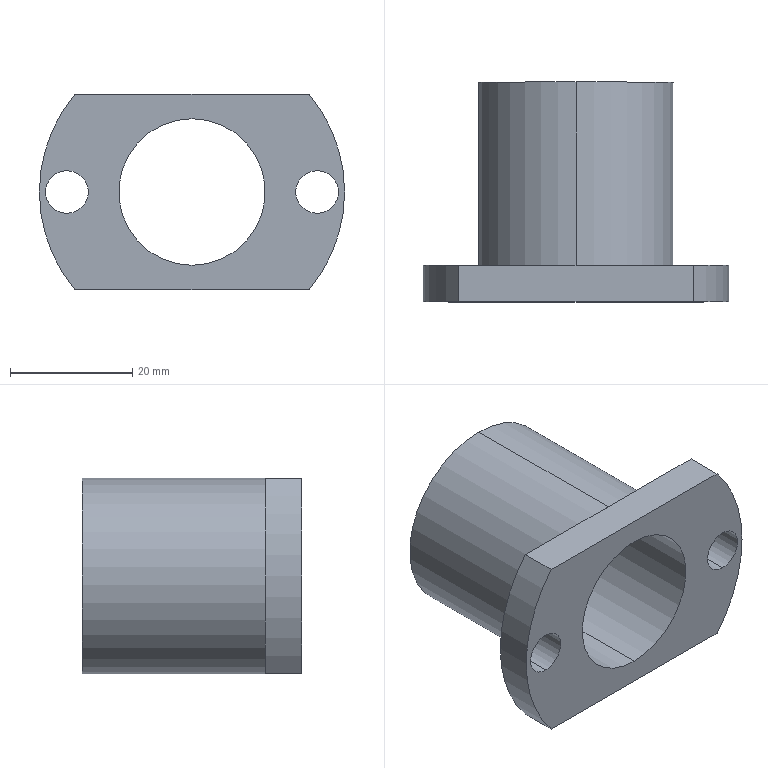Part | SolidWorks | features ICE 2, Revolution 1 | 1 solid | 16 faces | box 50 x 36 x 32 mm | volume 16277 mm3 | cylinder 10 | plane 6 | commonest cylinder face diameters 7 x4 24 x2 32 x2 50 x2
STEP:
#1=CARTESIAN_POINT('',(20.5,0.,-3.5));
#2=VERTEX_POINT('',#1);
#3=CARTESIAN_POINT('',(20.5,0.,3.5));
#4=VERTEX_POINT('',#3);
#5=CARTESIAN_POINT('',(20.5,0.,0.));
#6=DIRECTION('',(0.,1.,0.));
#7=DIRECTION('',(0.,0.,1.));
#8=AXIS2_PLACEMENT_3D('',#5,#6,#7);
#9=CIRCLE('',#8,3.5);
#10=EDGE_CURVE('',#2,#4,#9,.T.);
#11=ORIENTED_EDGE('',*,*,#10,.F.);
#12=CARTESIAN_POINT('',(20.5,6.,-3.5));
#13=VERTEX_POINT('',#12);
#14=CARTESIAN_POINT('',(20.5,0.,-3.5));
#15=DIRECTION('',(0.,1.,0.));
#16=VECTOR('',#15,1000.);
#17=LINE('',#14,#16);
#18=EDGE_CURVE('',#2,#13,#17,.T.);
#19=ORIENTED_EDGE('',*,*,#18,.T.);
#20=CARTESIAN_POINT('',(20.5,6.,3.5));
#21=VERTEX_POINT('',#20);
#22=CARTESIAN_POINT('',(20.5,6.,0.));
#23=DIRECTION('',(0.,1.,0.));
#24=DIRECTION('',(0.,0.,1.));
#25=AXIS2_PLACEMENT_3D('',#22,#23,#24);
#26=CIRCLE('',#25,3.5);
#27=EDGE_CURVE('',#13,#21,#26,.T.);
#28=ORIENTED_EDGE('',*,*,#27,.T.);
#29=CARTESIAN_POINT('',(20.5,0.,3.5));
#30=DIRECTION('',(0.,1.,0.));
#31=VECTOR('',#30,1000.);
#32=LINE('',#29,#31);
#33=EDGE_CURVE('',#4,#21,#32,.T.);
#34=ORIENTED_EDGE('',*,*,#33,.F.);
#35=EDGE_LOOP('',(#11,#19,#28,#34));
#36=FACE_OUTER_BOUND('',#35,.T.);
#37=CARTESIAN_POINT('',(20.5,0.,0.));
#38=DIRECTION('',(0.,1.,0.));
#39=DIRECTION('',(0.,0.,1.));
#40=AXIS2_PLACEMENT_3D('',#37,#38,#39);
#41=CYLINDRICAL_SURFACE('',#40,3.5);
#42=ADVANCED_FACE('',(#36),#41,.F.);
#43=CARTESIAN_POINT('',(-20.5,0.,-3.5));
#44=VERTEX_POINT('',#43);
#45=CARTESIAN_POINT('',(-20.5,0.,3.5));
#46=VERTEX_POINT('',#45);
#47=CARTESIAN_POINT('',(-20.5,0.,0.));
#48=DIRECTION('',(0.,1.,0.));
#49=DIRECTION('',(0.,0.,1.));
#50=AXIS2_PLACEMENT_3D('',#47,#48,#49);
#51=CIRCLE('',#50,3.5);
#52=EDGE_CURVE('',#44,#46,#51,.T.);
#53=ORIENTED_EDGE('',*,*,#52,.F.);
#54=CARTESIAN_POINT('',(-20.5,6.,-3.5));
#55=VERTEX_POINT('',#54);
#56=CARTESIAN_POINT('',(-20.5,0.,-3.5));
#57=DIRECTION('',(0.,1.,0.));
#58=VECTOR('',#57,1000.);
#59=LINE('',#56,#58);
#60=EDGE_CURVE('',#44,#55,#59,.T.);
#61=ORIENTED_EDGE('',*,*,#60,.T.);
#62=CARTESIAN_POINT('',(-20.5,6.,3.5));
#63=VERTEX_POINT('',#62);
#64=CARTESIAN_POINT('',(-20.5,6.,0.));
#65=DIRECTION('',(0.,1.,0.));
#66=DIRECTION('',(0.,0.,1.));
#67=AXIS2_PLACEMENT_3D('',#64,#65,#66);
#68=CIRCLE('',#67,3.5);
#69=EDGE_CURVE('',#55,#63,#68,.T.);
#70=ORIENTED_EDGE('',*,*,#69,.T.);
#71=CARTESIAN_POINT('',(-20.5,0.,3.5));
#72=DIRECTION('',(0.,1.,0.));
#73=VECTOR('',#72,1000.);
#74=LINE('',#71,#73);
#75=EDGE_CURVE('',#46,#63,#74,.T.);
#76=ORIENTED_EDGE('',*,*,#75,.F.);
#77=EDGE_LOOP('',(#53,#61,#70,#76));
#78=FACE_OUTER_BOUND('',#77,.T.);
#79=CARTESIAN_POINT('',(-20.5,0.,0.));
#80=DIRECTION('',(0.,1.,0.));
#81=DIRECTION('',(0.,0.,1.));
#82=AXIS2_PLACEMENT_3D('',#79,#80,#81);
#83=CYLINDRICAL_SURFACE('',#82,3.5);
#84=ADVANCED_FACE('',(#78),#83,.F.);
#85=CARTESIAN_POINT('',(0.,36.,-16.));
#86=VERTEX_POINT('',#85);
#87=CARTESIAN_POINT('',(0.,36.,16.));
#88=VERTEX_POINT('',#87);
#89=CARTESIAN_POINT('',(0.,36.,0.));
#90=DIRECTION('',(0.,-1.,0.));
#91=DIRECTION('',(0.,0.,-1.));
#92=AXIS2_PLACEMENT_3D('',#89,#90,#91);
#93=CIRCLE('',#92,16.);
#94=EDGE_CURVE('',#86,#88,#93,.T.);
#95=ORIENTED_EDGE('',*,*,#94,.T.);
#96=CARTESIAN_POINT('',(0.,6.,16.));
#97=VERTEX_POINT('',#96);
#98=CARTESIAN_POINT('',(0.,0.,16.));
#99=DIRECTION('',(0.,-1.,0.));
#100=VECTOR('',#99,1000.);
#101=LINE('',#98,#100);
#102=EDGE_CURVE('',#88,#97,#101,.T.);
#103=ORIENTED_EDGE('',*,*,#102,.T.);
#104=CARTESIAN_POINT('',(0.,6.,-16.));
#105=VERTEX_POINT('',#104);
#106=CARTESIAN_POINT('',(0.,6.,0.));
#107=DIRECTION('',(0.,-1.,0.));
#108=DIRECTION('',(0.,0.,-1.));
#109=AXIS2_PLACEMENT_3D('',#106,#107,#108);
#110=CIRCLE('',#109,16.);
#111=EDGE_CURVE('',#105,#97,#110,.T.);
#112=ORIENTED_EDGE('',*,*,#111,.F.);
#113=CARTESIAN_POINT('',(0.,0.,-16.));
#114=DIRECTION('',(0.,-1.,0.));
#115=VECTOR('',#114,1000.);
#116=LINE('',#113,#115);
#117=EDGE_CURVE('',#86,#105,#116,.T.);
#118=ORIENTED_EDGE('',*,*,#117,.F.);
#119=EDGE_LOOP('',(#95,#103,#112,#118));
#120=FACE_OUTER_BOUND('',#119,.T.);
#121=CARTESIAN_POINT('',(0.,0.,0.));
#122=DIRECTION('',(0.,-1.,0.));
#123=DIRECTION('',(0.,0.,-1.));
#124=AXIS2_PLACEMENT_3D('',#121,#122,#123);
#125=CYLINDRICAL_SURFACE('',#124,16.);
#126=ADVANCED_FACE('',(#120),#125,.T.);
#127=CARTESIAN_POINT('',(0.,36.,12.));
#128=VERTEX_POINT('',#127);
#129=CARTESIAN_POINT('',(0.,36.,-12.));
#130=VERTEX_POINT('',#129);
#131=CARTESIAN_POINT('',(0.,36.,0.));
#132=DIRECTION('',(0.,-1.,0.));
#133=DIRECTION('',(0.,0.,-1.));
#134=AXIS2_PLACEMENT_3D('',#131,#132,#133);
#135=CIRCLE('',#134,12.);
#136=EDGE_CURVE('',#128,#130,#135,.T.);
#137=ORIENTED_EDGE('',*,*,#136,.F.);
#138=CARTESIAN_POINT('',(0.,0.,12.));
#139=VERTEX_POINT('',#138);
#140=CARTESIAN_POINT('',(0.,0.,12.));
#141=DIRECTION('',(0.,-1.,0.));
#142=VECTOR('',#141,1000.);
#143=LINE('',#140,#142);
#144=EDGE_CURVE('',#128,#139,#143,.T.);
#145=ORIENTED_EDGE('',*,*,#144,.T.);
#146=CARTESIAN_POINT('',(0.,0.,-12.));
#147=VERTEX_POINT('',#146);
#148=CARTESIAN_POINT('',(0.,0.,0.));
#149=DIRECTION('',(0.,-1.,0.));
#150=DIRECTION('',(0.,0.,-1.));
#151=AXIS2_PLACEMENT_3D('',#148,#149,#150);
#152=CIRCLE('',#151,12.);
#153=EDGE_CURVE('',#139,#147,#152,.T.);
#154=ORIENTED_EDGE('',*,*,#153,.T.);
#155=CARTESIAN_POINT('',(0.,0.,-12.));
#156=DIRECTION('',(0.,-1.,0.));
#157=VECTOR('',#156,1000.);
#158=LINE('',#155,#157);
#159=EDGE_CURVE('',#130,#147,#158,.T.);
#160=ORIENTED_EDGE('',*,*,#159,.F.);
#161=EDGE_LOOP('',(#137,#145,#154,#160));
#162=FACE_OUTER_BOUND('',#161,.T.);
#163=CARTESIAN_POINT('',(0.,0.,0.));
#164=DIRECTION('',(0.,-1.,0.));
#165=DIRECTION('',(0.,0.,-1.));
#166=AXIS2_PLACEMENT_3D('',#163,#164,#165);
#167=CYLINDRICAL_SURFACE('',#166,12.);
#168=ADVANCED_FACE('',(#162),#167,.F.);
#169=CARTESIAN_POINT('',(19.209,0.,16.));
#170=VERTEX_POINT('',#169);
#171=CARTESIAN_POINT('',(19.209,6.,16.));
#172=VERTEX_POINT('',#171);
#173=CARTESIAN_POINT('',(19.209,0.,16.));
#174=DIRECTION('',(0.,1.,0.));
#175=VECTOR('',#174,1000.);
#176=LINE('',#173,#175);
#177=EDGE_CURVE('',#170,#172,#176,.T.);
#178=ORIENTED_EDGE('',*,*,#177,.F.);
#179=CARTESIAN_POINT('',(19.209,0.,-16.));
#180=VERTEX_POINT('',#179);
#181=CARTESIAN_POINT('',(0.,0.,0.));
#182=DIRECTION('',(0.,-1.,0.));
#183=DIRECTION('',(0.,0.,-1.));
#184=AXIS2_PLACEMENT_3D('',#181,#182,#183);
#185=CIRCLE('',#184,25.);
#186=EDGE_CURVE('',#180,#170,#185,.T.);
#187=ORIENTED_EDGE('',*,*,#186,.F.);
#188=CARTESIAN_POINT('',(19.209,6.,-16.));
#189=VERTEX_POINT('',#188);
#190=CARTESIAN_POINT('',(19.209,0.,-16.));
#191=DIRECTION('',(0.,1.,0.));
#192=VECTOR('',#191,1000.);
#193=LINE('',#190,#192);
#194=EDGE_CURVE('',#180,#189,#193,.T.);
#195=ORIENTED_EDGE('',*,*,#194,.T.);
#196=CARTESIAN_POINT('',(0.,6.,0.));
#197=DIRECTION('',(0.,-1.,0.));
#198=DIRECTION('',(0.,0.,-1.));
#199=AXIS2_PLACEMENT_3D('',#196,#197,#198);
#200=CIRCLE('',#199,25.);
#201=EDGE_CURVE('',#189,#172,#200,.T.);
#202=ORIENTED_EDGE('',*,*,#201,.T.);
#203=EDGE_LOOP('',(#178,#187,#195,#202));
#204=FACE_OUTER_BOUND('',#203,.T.);
#205=CARTESIAN_POINT('',(0.,0.,0.));
#206=DIRECTION('',(0.,-1.,0.));
#207=DIRECTION('',(0.,0.,-1.));
#208=AXIS2_PLACEMENT_3D('',#205,#206,#207);
#209=CYLINDRICAL_SURFACE('',#208,25.);
#210=ADVANCED_FACE('',(#204),#209,.T.);
#211=CARTESIAN_POINT('',(-19.209,6.,16.));
#212=DIRECTION('',(-1.,0.,0.));
#213=VECTOR('',#212,1000.);
#214=LINE('',#211,#213);
#215=EDGE_CURVE('',#172,#97,#214,.T.);
#216=ORIENTED_EDGE('',*,*,#215,.F.);
#217=ORIENTED_EDGE('',*,*,#201,.F.);
#218=CARTESIAN_POINT('',(-19.209,6.,-16.));
#219=DIRECTION('',(1.,0.,0.));
#220=VECTOR('',#219,1000.);
#221=LINE('',#218,#220);
#222=EDGE_CURVE('',#105,#189,#221,.T.);
#223=ORIENTED_EDGE('',*,*,#222,.F.);
#224=ORIENTED_EDGE('',*,*,#111,.T.);
#225=EDGE_LOOP('',(#216,#217,#223,#224));
#226=FACE_OUTER_BOUND('',#225,.T.);
#227=CARTESIAN_POINT('',(20.5,6.,0.));
#228=DIRECTION('',(0.,1.,0.));
#229=DIRECTION('',(0.,0.,1.));
#230=AXIS2_PLACEMENT_3D('',#227,#228,#229);
#231=CIRCLE('',#230,3.5);
#232=EDGE_CURVE('',#21,#13,#231,.T.);
#233=ORIENTED_EDGE('',*,*,#232,.F.);
#234=ORIENTED_EDGE('',*,*,#27,.F.);
#235=EDGE_LOOP('',(#233,#234));
#236=FACE_BOUND('',#235,.T.);
#237=CARTESIAN_POINT('',(25.,6.,0.));
#238=DIRECTION('',(0.,1.,0.));
#239=DIRECTION('',(0.,0.,1.));
#240=AXIS2_PLACEMENT_3D('',#237,#238,#239);
#241=PLANE('',#240);
#242=ADVANCED_FACE('',(#226,#236),#241,.T.);
#243=CARTESIAN_POINT('',(0.,36.,0.));
#244=DIRECTION('',(0.,-1.,0.));
#245=DIRECTION('',(0.,0.,-1.));
#246=AXIS2_PLACEMENT_3D('',#243,#244,#245);
#247=CIRCLE('',#246,12.);
#248=EDGE_CURVE('',#130,#128,#247,.T.);
#249=ORIENTED_EDGE('',*,*,#248,.T.);
#250=ORIENTED_EDGE('',*,*,#136,.T.);
#251=EDGE_LOOP('',(#249,#250));
#252=FACE_BOUND('',#251,.T.);
#253=ORIENTED_EDGE('',*,*,#94,.F.);
#254=CARTESIAN_POINT('',(0.,36.,0.));
#255=DIRECTION('',(0.,-1.,0.));
#256=DIRECTION('',(0.,0.,-1.));
#257=AXIS2_PLACEMENT_3D('',#254,#255,#256);
#258=CIRCLE('',#257,16.);
#259=EDGE_CURVE('',#88,#86,#258,.T.);
#260=ORIENTED_EDGE('',*,*,#259,.F.);
#261=EDGE_LOOP('',(#253,#260));
#262=FACE_OUTER_BOUND('',#261,.T.);
#263=CARTESIAN_POINT('',(16.,36.,0.));
#264=DIRECTION('',(0.,1.,0.));
#265=DIRECTION('',(0.,0.,1.));
#266=AXIS2_PLACEMENT_3D('',#263,#264,#265);
#267=PLANE('',#266);
#268=ADVANCED_FACE('',(#252,#262),#267,.T.);
#269=ORIENTED_EDGE('',*,*,#144,.F.);
#270=ORIENTED_EDGE('',*,*,#248,.F.);
#271=ORIENTED_EDGE('',*,*,#159,.T.);
#272=CARTESIAN_POINT('',(0.,0.,0.));
#273=DIRECTION('',(0.,-1.,0.));
#274=DIRECTION('',(0.,0.,-1.));
#275=AXIS2_PLACEMENT_3D('',#272,#273,#274);
#276=CIRCLE('',#275,12.);
#277=EDGE_CURVE('',#147,#139,#276,.T.);
#278=ORIENTED_EDGE('',*,*,#277,.T.);
#279=EDGE_LOOP('',(#269,#270,#271,#278));
#280=FACE_OUTER_BOUND('',#279,.T.);
#281=CARTESIAN_POINT('',(0.,0.,0.));
#282=DIRECTION('',(0.,-1.,0.));
#283=DIRECTION('',(0.,0.,-1.));
#284=AXIS2_PLACEMENT_3D('',#281,#282,#283);
#285=CYLINDRICAL_SURFACE('',#284,12.);
#286=ADVANCED_FACE('',(#280),#285,.F.);
#287=CARTESIAN_POINT('',(-19.209,0.,16.));
#288=VERTEX_POINT('',#287);
#289=CARTESIAN_POINT('',(-19.209,0.,16.));
#290=DIRECTION('',(-1.,0.,0.));
#291=VECTOR('',#290,1000.);
#292=LINE('',#289,#291);
#293=EDGE_CURVE('',#170,#288,#292,.T.);
#294=ORIENTED_EDGE('',*,*,#293,.T.);
#295=CARTESIAN_POINT('',(-19.209,0.,-16.));
#296=VERTEX_POINT('',#295);
#297=CARTESIAN_POINT('',(0.,0.,0.));
#298=DIRECTION('',(0.,-1.,0.));
#299=DIRECTION('',(0.,0.,-1.));
#300=AXIS2_PLACEMENT_3D('',#297,#298,#299);
#301=CIRCLE('',#300,25.);
#302=EDGE_CURVE('',#288,#296,#301,.T.);
#303=ORIENTED_EDGE('',*,*,#302,.T.);
#304=CARTESIAN_POINT('',(-19.209,0.,-16.));
#305=DIRECTION('',(1.,0.,0.));
#306=VECTOR('',#305,1000.);
#307=LINE('',#304,#306);
#308=EDGE_CURVE('',#296,#180,#307,.T.);
#309=ORIENTED_EDGE('',*,*,#308,.T.);
#310=ORIENTED_EDGE('',*,*,#186,.T.);
#311=EDGE_LOOP('',(#294,#303,#309,#310));
#312=FACE_OUTER_BOUND('',#311,.T.);
#313=CARTESIAN_POINT('',(20.5,0.,0.));
#314=DIRECTION('',(0.,1.,0.));
#315=DIRECTION('',(0.,0.,1.));
#316=AXIS2_PLACEMENT_3D('',#313,#314,#315);
#317=CIRCLE('',#316,3.5);
#318=EDGE_CURVE('',#4,#2,#317,.T.);
#319=ORIENTED_EDGE('',*,*,#318,.T.);
#320=ORIENTED_EDGE('',*,*,#10,.T.);
#321=EDGE_LOOP('',(#319,#320));
#322=FACE_BOUND('',#321,.T.);
#323=CARTESIAN_POINT('',(-20.5,0.,0.));
#324=DIRECTION('',(0.,1.,0.));
#325=DIRECTION('',(0.,0.,1.));
#326=AXIS2_PLACEMENT_3D('',#323,#324,#325);
#327=CIRCLE('',#326,3.5);
#328=EDGE_CURVE('',#46,#44,#327,.T.);
#329=ORIENTED_EDGE('',*,*,#328,.T.);
#330=ORIENTED_EDGE('',*,*,#52,.T.);
#331=EDGE_LOOP('',(#329,#330));
#332=FACE_BOUND('',#331,.T.);
#333=ORIENTED_EDGE('',*,*,#277,.F.);
#334=ORIENTED_EDGE('',*,*,#153,.F.);
#335=EDGE_LOOP('',(#333,#334));
#336=FACE_BOUND('',#335,.T.);
#337=CARTESIAN_POINT('',(12.,0.,0.));
#338=DIRECTION('',(0.,-1.,0.));
#339=DIRECTION('',(0.,0.,-1.));
#340=AXIS2_PLACEMENT_3D('',#337,#338,#339);
#341=PLANE('',#340);
#342=ADVANCED_FACE('',(#312,#322,#332,#336),#341,.T.);
#343=CARTESIAN_POINT('',(-19.209,6.,16.));
#344=VERTEX_POINT('',#343);
#345=CARTESIAN_POINT('',(-19.209,0.,16.));
#346=DIRECTION('',(0.,1.,0.));
#347=VECTOR('',#346,1000.);
#348=LINE('',#345,#347);
#349=EDGE_CURVE('',#288,#344,#348,.T.);
#350=ORIENTED_EDGE('',*,*,#349,.T.);
#351=CARTESIAN_POINT('',(-19.209,6.,-16.));
#352=VERTEX_POINT('',#351);
#353=CARTESIAN_POINT('',(0.,6.,0.));
#354=DIRECTION('',(0.,-1.,0.));
#355=DIRECTION('',(0.,0.,-1.));
#356=AXIS2_PLACEMENT_3D('',#353,#354,#355);
#357=CIRCLE('',#356,25.);
#358=EDGE_CURVE('',#344,#352,#357,.T.);
#359=ORIENTED_EDGE('',*,*,#358,.T.);
#360=CARTESIAN_POINT('',(-19.209,0.,-16.));
#361=DIRECTION('',(0.,1.,0.));
#362=VECTOR('',#361,1000.);
#363=LINE('',#360,#362);
#364=EDGE_CURVE('',#296,#352,#363,.T.);
#365=ORIENTED_EDGE('',*,*,#364,.F.);
#366=ORIENTED_EDGE('',*,*,#302,.F.);
#367=EDGE_LOOP('',(#350,#359,#365,#366));
#368=FACE_OUTER_BOUND('',#367,.T.);
#369=CARTESIAN_POINT('',(0.,0.,0.));
#370=DIRECTION('',(0.,-1.,0.));
#371=DIRECTION('',(0.,0.,-1.));
#372=AXIS2_PLACEMENT_3D('',#369,#370,#371);
#373=CYLINDRICAL_SURFACE('',#372,25.);
#374=ADVANCED_FACE('',(#368),#373,.T.);
#375=CARTESIAN_POINT('',(-19.209,6.,16.));
#376=DIRECTION('',(-1.,0.,0.));
#377=VECTOR('',#376,1000.);
#378=LINE('',#375,#377);
#379=EDGE_CURVE('',#97,#344,#378,.T.);
#380=ORIENTED_EDGE('',*,*,#379,.F.);
#381=CARTESIAN_POINT('',(0.,6.,0.));
#382=DIRECTION('',(0.,-1.,0.));
#383=DIRECTION('',(0.,0.,-1.));
#384=AXIS2_PLACEMENT_3D('',#381,#382,#383);
#385=CIRCLE('',#384,16.);
#386=EDGE_CURVE('',#97,#105,#385,.T.);
#387=ORIENTED_EDGE('',*,*,#386,.T.);
#388=CARTESIAN_POINT('',(-19.209,6.,-16.));
#389=DIRECTION('',(1.,0.,0.));
#390=VECTOR('',#389,1000.);
#391=LINE('',#388,#390);
#392=EDGE_CURVE('',#352,#105,#391,.T.);
#393=ORIENTED_EDGE('',*,*,#392,.F.);
#394=ORIENTED_EDGE('',*,*,#358,.F.);
#395=EDGE_LOOP('',(#380,#387,#393,#394));
#396=FACE_OUTER_BOUND('',#395,.T.);
#397=CARTESIAN_POINT('',(-20.5,6.,0.));
#398=DIRECTION('',(0.,1.,0.));
#399=DIRECTION('',(0.,0.,1.));
#400=AXIS2_PLACEMENT_3D('',#397,#398,#399);
#401=CIRCLE('',#400,3.5);
#402=EDGE_CURVE('',#63,#55,#401,.T.);
#403=ORIENTED_EDGE('',*,*,#402,.F.);
#404=ORIENTED_EDGE('',*,*,#69,.F.);
#405=EDGE_LOOP('',(#403,#404));
#406=FACE_BOUND('',#405,.T.);
#407=CARTESIAN_POINT('',(25.,6.,0.));
#408=DIRECTION('',(0.,1.,0.));
#409=DIRECTION('',(0.,0.,1.));
#410=AXIS2_PLACEMENT_3D('',#407,#408,#409);
#411=PLANE('',#410);
#412=ADVANCED_FACE('',(#396,#406),#411,.T.);
#413=ORIENTED_EDGE('',*,*,#102,.F.);
#414=ORIENTED_EDGE('',*,*,#259,.T.);
#415=ORIENTED_EDGE('',*,*,#117,.T.);
#416=ORIENTED_EDGE('',*,*,#386,.F.);
#417=EDGE_LOOP('',(#413,#414,#415,#416));
#418=FACE_OUTER_BOUND('',#417,.T.);
#419=CARTESIAN_POINT('',(0.,0.,0.));
#420=DIRECTION('',(0.,-1.,0.));
#421=DIRECTION('',(0.,0.,-1.));
#422=AXIS2_PLACEMENT_3D('',#419,#420,#421);
#423=CYLINDRICAL_SURFACE('',#422,16.);
#424=ADVANCED_FACE('',(#418),#423,.T.);
#425=ORIENTED_EDGE('',*,*,#60,.F.);
#426=ORIENTED_EDGE('',*,*,#328,.F.);
#427=ORIENTED_EDGE('',*,*,#75,.T.);
#428=ORIENTED_EDGE('',*,*,#402,.T.);
#429=EDGE_LOOP('',(#425,#426,#427,#428));
#430=FACE_OUTER_BOUND('',#429,.T.);
#431=CARTESIAN_POINT('',(-20.5,0.,0.));
#432=DIRECTION('',(0.,1.,0.));
#433=DIRECTION('',(0.,0.,1.));
#434=AXIS2_PLACEMENT_3D('',#431,#432,#433);
#435=CYLINDRICAL_SURFACE('',#434,3.5);
#436=ADVANCED_FACE('',(#430),#435,.F.);
#437=ORIENTED_EDGE('',*,*,#18,.F.);
#438=ORIENTED_EDGE('',*,*,#318,.F.);
#439=ORIENTED_EDGE('',*,*,#33,.T.);
#440=ORIENTED_EDGE('',*,*,#232,.T.);
#441=EDGE_LOOP('',(#437,#438,#439,#440));
#442=FACE_OUTER_BOUND('',#441,.T.);
#443=CARTESIAN_POINT('',(20.5,0.,0.));
#444=DIRECTION('',(0.,1.,0.));
#445=DIRECTION('',(0.,0.,1.));
#446=AXIS2_PLACEMENT_3D('',#443,#444,#445);
#447=CYLINDRICAL_SURFACE('',#446,3.5);
#448=ADVANCED_FACE('',(#442),#447,.F.);
#449=ORIENTED_EDGE('',*,*,#392,.T.);
#450=ORIENTED_EDGE('',*,*,#222,.T.);
#451=ORIENTED_EDGE('',*,*,#194,.F.);
#452=ORIENTED_EDGE('',*,*,#308,.F.);
#453=ORIENTED_EDGE('',*,*,#364,.T.);
#454=EDGE_LOOP('',(#449,#450,#451,#452,#453));
#455=FACE_OUTER_BOUND('',#454,.T.);
#456=CARTESIAN_POINT('',(-19.209,0.,-16.));
#457=DIRECTION('',(0.,0.,1.));
#458=DIRECTION('',(1.,0.,0.));
#459=AXIS2_PLACEMENT_3D('',#456,#457,#458);
#460=PLANE('',#459);
#461=ADVANCED_FACE('',(#455),#460,.F.);
#462=ORIENTED_EDGE('',*,*,#215,.T.);
#463=ORIENTED_EDGE('',*,*,#379,.T.);
#464=ORIENTED_EDGE('',*,*,#349,.F.);
#465=ORIENTED_EDGE('',*,*,#293,.F.);
#466=ORIENTED_EDGE('',*,*,#177,.T.);
#467=EDGE_LOOP('',(#462,#463,#464,#465,#466));
#468=FACE_OUTER_BOUND('',#467,.T.);
#469=CARTESIAN_POINT('',(-19.209,0.,16.));
#470=DIRECTION('',(0.,0.,-1.));
#471=DIRECTION('',(-1.,0.,0.));
#472=AXIS2_PLACEMENT_3D('',#469,#470,#471);
#473=PLANE('',#472);
#474=ADVANCED_FACE('',(#468),#473,.F.);
#475=CLOSED_SHELL('',(#42,#84,#126,#168,#210,#242,#268,#286,#342,#374,#412,#424,#436,#448,#461,#474));
#476=MANIFOLD_SOLID_BREP('',#475);
#477=CARTESIAN_POINT('',(0.,0.,0.));
#478=DIRECTION('',(0.,0.,1.));
#479=DIRECTION('',(1.,0.,0.));
#480=AXIS2_PLACEMENT_3D('',#477,#478,#479);
#481=(LENGTH_UNIT()NAMED_UNIT(*)SI_UNIT(.MILLI.,.METRE.));
#482=UNCERTAINTY_MEASURE_WITH_UNIT(LENGTH_MEASURE(0.00001),#481,'','');
#483=(NAMED_UNIT(*)PLANE_ANGLE_UNIT()SI_UNIT($,.RADIAN.));
#484=(NAMED_UNIT(*)SI_UNIT($,.STERADIAN.)SOLID_ANGLE_UNIT());
#485=(GEOMETRIC_REPRESENTATION_CONTEXT(3)GLOBAL_UNCERTAINTY_ASSIGNED_CONTEXT((#482))GLOBAL_UNIT_ASSIGNED_CONTEXT((#481,#483,#484))REPRESENTATION_CONTEXT('',''));
#486=ADVANCED_BREP_SHAPE_REPRESENTATION('',(#476,#480),#485);